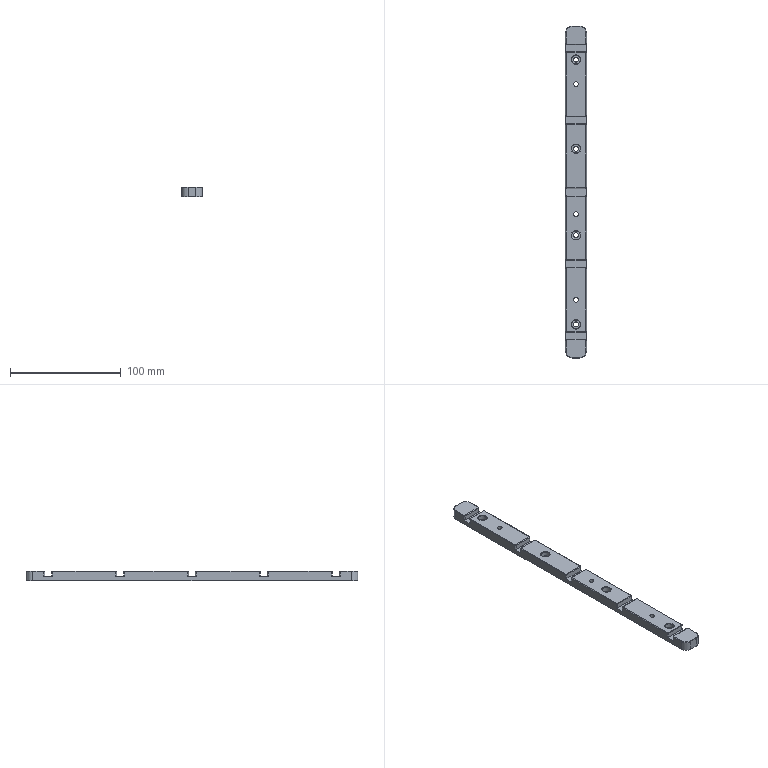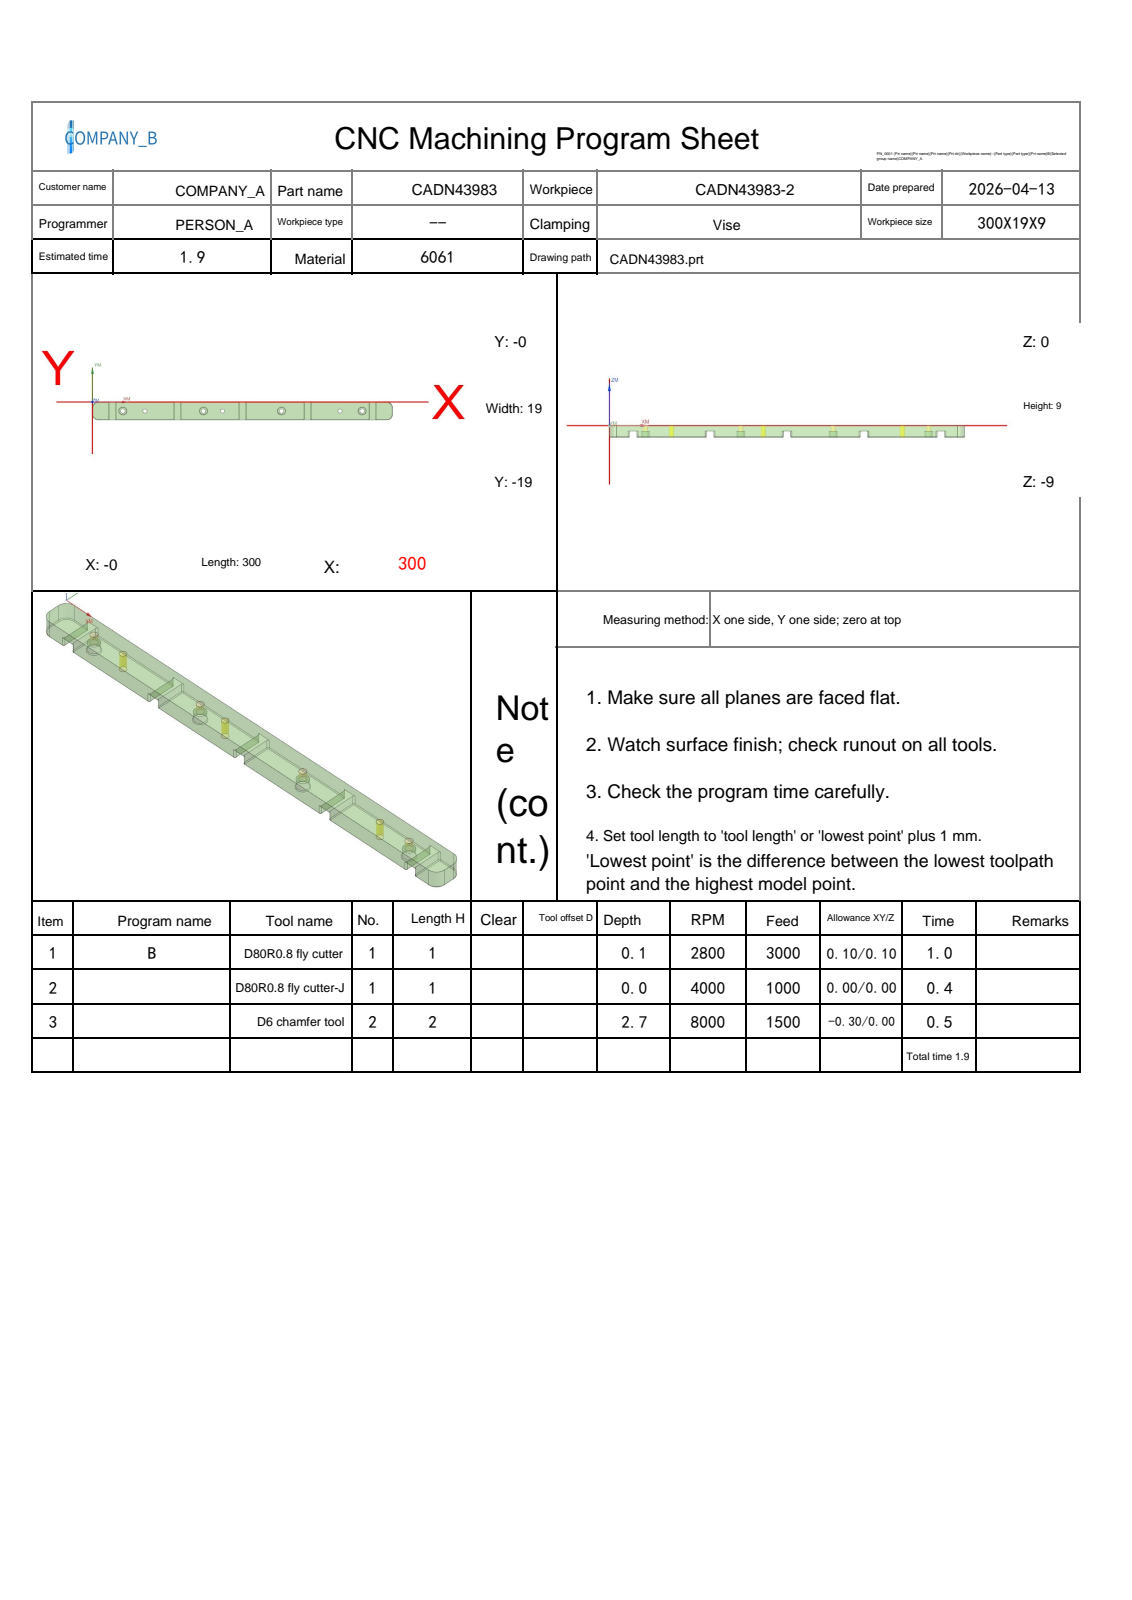NC program | NX | posted by the shop | part box 19 x 300 x 9 mm
Whole program:
%
O0001
(Machine time: 2.55 MIN)
(===Total Tool:2===)
(T1=D80R0.8 fly cutter D=80.  R=0.8  D-  H01 Z=-0.   )
(T2=D6 chamfer tool   D=6.   R=0.   D-  H02 Z=-2.7  )
G80 G90 G17 G49 G40
G91 G28 Z0
M01
N1 T01 M06
(D80R0.8 fly cutter  D=80. R=0.8 H=01 ce=0.10 di=0.10)
G00 G90 G54 X-52.097 Y-12.165 M03 S2800
G43 H01 Z20.
M08
Z4.517
G01 Z2.517 F3000.
X-40.097 Y-12.007
X340.097 Y-6.993
X352.097 Y-6.835
Z4.517
G00 X-52.097 Y-12.165
Z4.033
G01 Z2.033
X-40.097 Y-12.007
X340.097 Y-6.993
X352.097 Y-6.835
Z4.033
G00 X-52.097 Y-12.165
Z3.55
G01 Z1.55
X-40.097 Y-12.007
X340.097 Y-6.993
X352.097 Y-6.835
Z3.55
G00 X-52.097 Y-12.165
Z3.067
G01 Z1.067
X-40.097 Y-12.007
X340.097 Y-6.993
X352.097 Y-6.835
Z3.067
G00 Z20.
X-52.097 Y-12.165
Z2.583
G01 Z.583
X-40.097 Y-12.007
X340.097 Y-6.993
X352.097 Y-6.835
Z2.583
G00 Z20.
X-52.097 Y-12.165
Z2.1
G01 Z.1
X-40.097 Y-12.007
X340.097 Y-6.993
X352.097 Y-6.835
Z2.1
G00 Z20.
G91 G28 Z0.0
M05
M09
G91 G28 Z0.0
M01
N2 T01 M06
(D80R0.8 fly cutter-J  D=80. R=0.8 H=01 ce=0.00 di=0.00)
G00 G90 G54 X-51.999 Y-12.158 M03 S4000
G43 H01 Z20.
M08
Z2.
G01 Z0.0 F1000.
X-39.999 Y-12.
X339.999 Y-7.
X351.999 Y-6.842
Z2.
G00 Z20.
G91 G28 Z0.0
M05
M09
G91 G28 Z0.0
M01
N3 T02 M06
(D6 chamfer tool  D=6. R=0. H=02 ce=0.00 di=0.00)
G00 G90 G54 X247.5 Y-9.5 M03 S8000
G43 H02 Z20.
M08
G98 G81 X247.5 Y-9.5 Z-2.7 R3. F1000.
X130.
X52.5
G80
G00 Z20.
G00 G90 X269.6 Y-9.5 M03 S8000
Z20.
G98 G81 X269.6 Y-9.5 Z-2.55 R3. F1000.
X189.
X111.
X30.4
G80
G00 Z20.
G00 G90 X300.194 Y-3.451 M03 S7000
Z20.
Z2.5
G01 X300.26 Y-3.603 Z2.44 F1500.
X300.439 Y-4.136 Z2.235
X300.572 Y-4.683 Z2.03
X300.66 Y-5.238 Z1.826
X300.7 Y-5.799 Z1.621
Y-13. Z-1.
G02 X294. Y-19.7 I-6.7 J0.0
G01 X6.
G02 X-.7 Y-13. I0.0 J6.7
G01 Y-6.
G02 X6. Y.7 I6.7 J0.0
G01 X294.
G02 X300.7 Y-6. I0.0 J-6.7
G01 Y-13.
G02 X300.681 Y-13.5 I-6.7 J0.0
G01 Z1.5
G00 Z20.
M05
M09
G91 G28 Z0.0
G91 G28 Y0.0
M30
%